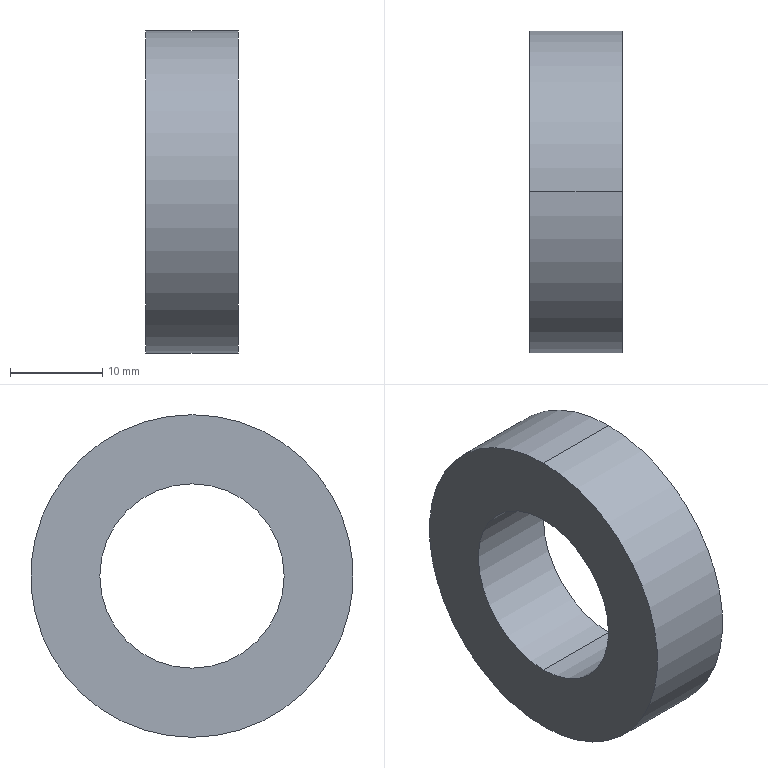Part | STEP file | urws35_20_10_2_03 | 1 solid | 6 faces | box 10 x 35 x 35 mm | volume 6480 mm3 | cylinder 4 | plane 2 | commonest cylinder face diameters 20 x2 35 x2
STEP:
#1=CARTESIAN_POINT('',(0.,0.,0.));
#2=DIRECTION('',(0.,0.,1.));
#3=DIRECTION('',(1.,0.,0.));
#4=AXIS2_PLACEMENT_3D('',#1,#2,#3);
#5=CARTESIAN_POINT('',(0.,0.,-17.5));
#6=VERTEX_POINT('',#5);
#7=CARTESIAN_POINT('',(0.,0.,17.5));
#8=VERTEX_POINT('',#7);
#9=CARTESIAN_POINT('',(0.,0.,0.));
#10=DIRECTION('',(1.,0.,0.));
#11=DIRECTION('',(0.,0.,-1.));
#12=AXIS2_PLACEMENT_3D('',#9,#10,#11);
#13=CIRCLE('',#12,17.5);
#14=CARTESIAN_POINT('',(5.,0.,0.));
#15=DIRECTION('',(1.,0.,0.));
#16=DIRECTION('',(0.,0.,-1.));
#17=AXIS2_PLACEMENT_3D('',#14,#15,#16);
#18=CYLINDRICAL_SURFACE('',#17,17.5);
#19=CARTESIAN_POINT('',(0.,-5.));
#20=DIRECTION('',(1.,0.));
#21=VECTOR('',#20,1.);
#22=LINE('',#19,#21);
#23=(GEOMETRIC_REPRESENTATION_CONTEXT(2)PARAMETRIC_REPRESENTATION_CONTEXT()REPRESENTATION_CONTEXT('',''));
#24=DEFINITIONAL_REPRESENTATION('',(#22),#23);
#25=PCURVE('',#18,#24);
#26=CARTESIAN_POINT('',(0.,8.75,0.));
#27=DIRECTION('',(-1.,0.,0.));
#28=DIRECTION('',(0.,0.,1.));
#29=AXIS2_PLACEMENT_3D('',#26,#27,#28);
#30=PLANE('',#29);
#31=CARTESIAN_POINT('',(-17.5,-8.75));
#32=CARTESIAN_POINT('',(-17.5,21.561));
#33=CARTESIAN_POINT('',(8.75,6.405));
#34=CARTESIAN_POINT('',(35.,-8.75));
#35=CARTESIAN_POINT('',(8.75,-23.905));
#36=CARTESIAN_POINT('',(-17.5,-39.061));
#37=CARTESIAN_POINT('',(-17.5,-8.75));
#38=(BOUNDED_CURVE()B_SPLINE_CURVE(2,(#31,#32,#33,#34,#35,#36,#37),.UNSPECIFIED.,.T.,.F.)B_SPLINE_CURVE_WITH_KNOTS((1,2,2,2,2,1),(-2.094,0.,2.094,4.189,6.283,8.378),.UNSPECIFIED.)CURVE()GEOMETRIC_REPRESENTATION_ITEM()RATIONAL_B_SPLINE_CURVE((1.,0.5,1.,0.5,1.,0.5,1.))REPRESENTATION_ITEM(''));
#39=(GEOMETRIC_REPRESENTATION_CONTEXT(2)PARAMETRIC_REPRESENTATION_CONTEXT()REPRESENTATION_CONTEXT('',''));
#40=DEFINITIONAL_REPRESENTATION('',(#38),#39);
#41=PCURVE('',#30,#40);
#42=SURFACE_CURVE('',#13,(#25,#41),.PCURVE_S1.);
#43=EDGE_CURVE('',#6,#8,#42,.T.);
#44=ORIENTED_EDGE('',*,*,#43,.T.);
#45=CARTESIAN_POINT('',(10.,0.,17.5));
#46=VERTEX_POINT('',#45);
#47=CARTESIAN_POINT('',(5.,0.,17.5));
#48=DIRECTION('',(1.,0.,0.));
#49=VECTOR('',#48,1.);
#50=LINE('',#47,#49);
#51=CARTESIAN_POINT('',(3.142,0.));
#52=DIRECTION('',(0.,1.));
#53=VECTOR('',#52,1.);
#54=LINE('',#51,#53);
#55=(GEOMETRIC_REPRESENTATION_CONTEXT(2)PARAMETRIC_REPRESENTATION_CONTEXT()REPRESENTATION_CONTEXT('',''));
#56=DEFINITIONAL_REPRESENTATION('',(#54),#55);
#57=PCURVE('',#18,#56);
#58=CARTESIAN_POINT('',(5.,0.,0.));
#59=DIRECTION('',(1.,0.,0.));
#60=DIRECTION('',(0.,0.,-1.));
#61=AXIS2_PLACEMENT_3D('',#58,#59,#60);
#62=CYLINDRICAL_SURFACE('',#61,17.5);
#63=CARTESIAN_POINT('',(3.142,0.));
#64=DIRECTION('',(0.,1.));
#65=VECTOR('',#64,1.);
#66=LINE('',#63,#65);
#67=(GEOMETRIC_REPRESENTATION_CONTEXT(2)PARAMETRIC_REPRESENTATION_CONTEXT()REPRESENTATION_CONTEXT('',''));
#68=DEFINITIONAL_REPRESENTATION('',(#66),#67);
#69=PCURVE('',#62,#68);
#70=SURFACE_CURVE('',#50,(#57,#69),.PCURVE_S1.);
#71=EDGE_CURVE('',#8,#46,#70,.T.);
#72=ORIENTED_EDGE('',*,*,#71,.T.);
#73=CARTESIAN_POINT('',(10.,0.,-17.5));
#74=VERTEX_POINT('',#73);
#75=CARTESIAN_POINT('',(10.,0.,0.));
#76=DIRECTION('',(1.,0.,0.));
#77=DIRECTION('',(0.,0.,-1.));
#78=AXIS2_PLACEMENT_3D('',#75,#76,#77);
#79=CIRCLE('',#78,17.5);
#80=CARTESIAN_POINT('',(0.,5.));
#81=DIRECTION('',(1.,0.));
#82=VECTOR('',#81,1.);
#83=LINE('',#80,#82);
#84=(GEOMETRIC_REPRESENTATION_CONTEXT(2)PARAMETRIC_REPRESENTATION_CONTEXT()REPRESENTATION_CONTEXT('',''));
#85=DEFINITIONAL_REPRESENTATION('',(#83),#84);
#86=PCURVE('',#18,#85);
#87=CARTESIAN_POINT('',(10.,8.75,0.));
#88=DIRECTION('',(1.,0.,0.));
#89=DIRECTION('',(0.,0.,-1.));
#90=AXIS2_PLACEMENT_3D('',#87,#88,#89);
#91=PLANE('',#90);
#92=CARTESIAN_POINT('',(0.,-8.75));
#93=DIRECTION('',(1.,0.));
#94=AXIS2_PLACEMENT_2D('',#92,#93);
#95=CIRCLE('',#94,17.5);
#96=(GEOMETRIC_REPRESENTATION_CONTEXT(2)PARAMETRIC_REPRESENTATION_CONTEXT()REPRESENTATION_CONTEXT('',''));
#97=DEFINITIONAL_REPRESENTATION('',(#95),#96);
#98=PCURVE('',#91,#97);
#99=SURFACE_CURVE('',#79,(#86,#98),.PCURVE_S1.);
#100=EDGE_CURVE('',#74,#46,#99,.T.);
#101=ORIENTED_EDGE('',*,*,#100,.F.);
#102=CARTESIAN_POINT('',(5.,0.,-17.5));
#103=DIRECTION('',(1.,0.,0.));
#104=VECTOR('',#103,1.);
#105=LINE('',#102,#104);
#106=CARTESIAN_POINT('',(0.,0.));
#107=DIRECTION('',(0.,1.));
#108=VECTOR('',#107,1.);
#109=LINE('',#106,#108);
#110=(GEOMETRIC_REPRESENTATION_CONTEXT(2)PARAMETRIC_REPRESENTATION_CONTEXT()REPRESENTATION_CONTEXT('',''));
#111=DEFINITIONAL_REPRESENTATION('',(#109),#110);
#112=PCURVE('',#18,#111);
#113=CARTESIAN_POINT('',(6.283,0.));
#114=DIRECTION('',(0.,1.));
#115=VECTOR('',#114,1.);
#116=LINE('',#113,#115);
#117=(GEOMETRIC_REPRESENTATION_CONTEXT(2)PARAMETRIC_REPRESENTATION_CONTEXT()REPRESENTATION_CONTEXT('',''));
#118=DEFINITIONAL_REPRESENTATION('',(#116),#117);
#119=PCURVE('',#62,#118);
#120=SURFACE_CURVE('',#105,(#112,#119),.PCURVE_S1.);
#121=EDGE_CURVE('',#6,#74,#120,.T.);
#122=ORIENTED_EDGE('',*,*,#121,.F.);
#123=EDGE_LOOP('',(#44,#72,#101,#122));
#124=FACE_BOUND('',#123,.T.);
#125=ADVANCED_FACE('',(#124),#18,.T.);
#126=CARTESIAN_POINT('',(10.,0.,10.));
#127=VERTEX_POINT('',#126);
#128=CARTESIAN_POINT('',(0.,0.,10.));
#129=VERTEX_POINT('',#128);
#130=CARTESIAN_POINT('',(0.,0.,10.));
#131=DIRECTION('',(-1.,0.,0.));
#132=VECTOR('',#131,1.);
#133=LINE('',#130,#132);
#134=CARTESIAN_POINT('',(0.,0.,0.));
#135=DIRECTION('',(-1.,0.,0.));
#136=DIRECTION('',(0.,0.,1.));
#137=AXIS2_PLACEMENT_3D('',#134,#135,#136);
#138=CYLINDRICAL_SURFACE('',#137,10.);
#139=CARTESIAN_POINT('',(6.283,0.));
#140=DIRECTION('',(0.,1.));
#141=VECTOR('',#140,1.);
#142=LINE('',#139,#141);
#143=(GEOMETRIC_REPRESENTATION_CONTEXT(2)PARAMETRIC_REPRESENTATION_CONTEXT()REPRESENTATION_CONTEXT('',''));
#144=DEFINITIONAL_REPRESENTATION('',(#142),#143);
#145=PCURVE('',#138,#144);
#146=CARTESIAN_POINT('',(0.,0.,0.));
#147=DIRECTION('',(-1.,0.,0.));
#148=DIRECTION('',(0.,0.,1.));
#149=AXIS2_PLACEMENT_3D('',#146,#147,#148);
#150=CYLINDRICAL_SURFACE('',#149,10.);
#151=CARTESIAN_POINT('',(0.,0.));
#152=DIRECTION('',(0.,1.));
#153=VECTOR('',#152,1.);
#154=LINE('',#151,#153);
#155=(GEOMETRIC_REPRESENTATION_CONTEXT(2)PARAMETRIC_REPRESENTATION_CONTEXT()REPRESENTATION_CONTEXT('',''));
#156=DEFINITIONAL_REPRESENTATION('',(#154),#155);
#157=PCURVE('',#150,#156);
#158=SURFACE_CURVE('',#133,(#145,#157),.PCURVE_S1.);
#159=EDGE_CURVE('',#127,#129,#158,.T.);
#160=ORIENTED_EDGE('',*,*,#159,.T.);
#161=CARTESIAN_POINT('',(0.,0.,-10.));
#162=VERTEX_POINT('',#161);
#163=CARTESIAN_POINT('',(0.,0.,0.));
#164=DIRECTION('',(1.,0.,0.));
#165=DIRECTION('',(0.,0.,1.));
#166=AXIS2_PLACEMENT_3D('',#163,#164,#165);
#167=CIRCLE('',#166,10.);
#168=CARTESIAN_POINT('',(6.283,0.));
#169=DIRECTION('',(-1.,0.));
#170=VECTOR('',#169,1.);
#171=LINE('',#168,#170);
#172=(GEOMETRIC_REPRESENTATION_CONTEXT(2)PARAMETRIC_REPRESENTATION_CONTEXT()REPRESENTATION_CONTEXT('',''));
#173=DEFINITIONAL_REPRESENTATION('',(#171),#172);
#174=PCURVE('',#138,#173);
#175=CARTESIAN_POINT('',(10.,-8.75));
#176=CARTESIAN_POINT('',(10.,-26.071));
#177=CARTESIAN_POINT('',(-5.,-17.41));
#178=CARTESIAN_POINT('',(-20.,-8.75));
#179=CARTESIAN_POINT('',(-5.,-0.08975));
#180=CARTESIAN_POINT('',(10.,8.571));
#181=CARTESIAN_POINT('',(10.,-8.75));
#182=(BOUNDED_CURVE()B_SPLINE_CURVE(2,(#175,#176,#177,#178,#179,#180,#181),.UNSPECIFIED.,.T.,.F.)B_SPLINE_CURVE_WITH_KNOTS((1,2,2,2,2,1),(-2.094,0.,2.094,4.189,6.283,8.378),.UNSPECIFIED.)CURVE()GEOMETRIC_REPRESENTATION_ITEM()RATIONAL_B_SPLINE_CURVE((1.,0.5,1.,0.5,1.,0.5,1.))REPRESENTATION_ITEM(''));
#183=(GEOMETRIC_REPRESENTATION_CONTEXT(2)PARAMETRIC_REPRESENTATION_CONTEXT()REPRESENTATION_CONTEXT('',''));
#184=DEFINITIONAL_REPRESENTATION('',(#182),#183);
#185=PCURVE('',#30,#184);
#186=SURFACE_CURVE('',#167,(#174,#185),.PCURVE_S1.);
#187=EDGE_CURVE('',#129,#162,#186,.T.);
#188=ORIENTED_EDGE('',*,*,#187,.T.);
#189=CARTESIAN_POINT('',(10.,0.,-10.));
#190=VERTEX_POINT('',#189);
#191=CARTESIAN_POINT('',(0.,0.,-10.));
#192=DIRECTION('',(-1.,0.,0.));
#193=VECTOR('',#192,1.);
#194=LINE('',#191,#193);
#195=CARTESIAN_POINT('',(3.142,0.));
#196=DIRECTION('',(0.,1.));
#197=VECTOR('',#196,1.);
#198=LINE('',#195,#197);
#199=(GEOMETRIC_REPRESENTATION_CONTEXT(2)PARAMETRIC_REPRESENTATION_CONTEXT()REPRESENTATION_CONTEXT('',''));
#200=DEFINITIONAL_REPRESENTATION('',(#198),#199);
#201=PCURVE('',#138,#200);
#202=CARTESIAN_POINT('',(3.142,0.));
#203=DIRECTION('',(0.,1.));
#204=VECTOR('',#203,1.);
#205=LINE('',#202,#204);
#206=(GEOMETRIC_REPRESENTATION_CONTEXT(2)PARAMETRIC_REPRESENTATION_CONTEXT()REPRESENTATION_CONTEXT('',''));
#207=DEFINITIONAL_REPRESENTATION('',(#205),#206);
#208=PCURVE('',#150,#207);
#209=SURFACE_CURVE('',#194,(#201,#208),.PCURVE_S1.);
#210=EDGE_CURVE('',#190,#162,#209,.T.);
#211=ORIENTED_EDGE('',*,*,#210,.F.);
#212=CARTESIAN_POINT('',(10.,0.,0.));
#213=DIRECTION('',(-1.,0.,0.));
#214=DIRECTION('',(0.,0.,1.));
#215=AXIS2_PLACEMENT_3D('',#212,#213,#214);
#216=CIRCLE('',#215,10.);
#217=CARTESIAN_POINT('',(0.,-10.));
#218=DIRECTION('',(1.,0.));
#219=VECTOR('',#218,1.);
#220=LINE('',#217,#219);
#221=(GEOMETRIC_REPRESENTATION_CONTEXT(2)PARAMETRIC_REPRESENTATION_CONTEXT()REPRESENTATION_CONTEXT('',''));
#222=DEFINITIONAL_REPRESENTATION('',(#220),#221);
#223=PCURVE('',#138,#222);
#224=CARTESIAN_POINT('',(-10.,-8.75));
#225=CARTESIAN_POINT('',(-10.,8.571));
#226=CARTESIAN_POINT('',(5.,-0.08975));
#227=CARTESIAN_POINT('',(20.,-8.75));
#228=CARTESIAN_POINT('',(5.,-17.41));
#229=CARTESIAN_POINT('',(-10.,-26.071));
#230=CARTESIAN_POINT('',(-10.,-8.75));
#231=(BOUNDED_CURVE()B_SPLINE_CURVE(2,(#224,#225,#226,#227,#228,#229,#230),.UNSPECIFIED.,.T.,.F.)B_SPLINE_CURVE_WITH_KNOTS((1,2,2,2,2,1),(-2.094,0.,2.094,4.189,6.283,8.378),.UNSPECIFIED.)CURVE()GEOMETRIC_REPRESENTATION_ITEM()RATIONAL_B_SPLINE_CURVE((1.,0.5,1.,0.5,1.,0.5,1.))REPRESENTATION_ITEM(''));
#232=(GEOMETRIC_REPRESENTATION_CONTEXT(2)PARAMETRIC_REPRESENTATION_CONTEXT()REPRESENTATION_CONTEXT('',''));
#233=DEFINITIONAL_REPRESENTATION('',(#231),#232);
#234=PCURVE('',#91,#233);
#235=SURFACE_CURVE('',#216,(#223,#234),.PCURVE_S1.);
#236=EDGE_CURVE('',#190,#127,#235,.T.);
#237=ORIENTED_EDGE('',*,*,#236,.T.);
#238=EDGE_LOOP('',(#160,#188,#211,#237));
#239=FACE_BOUND('',#238,.F.);
#240=ADVANCED_FACE('',(#239),#138,.F.);
#241=ORIENTED_EDGE('',*,*,#100,.T.);
#242=CARTESIAN_POINT('',(10.,0.,0.));
#243=DIRECTION('',(1.,0.,0.));
#244=DIRECTION('',(0.,0.,-1.));
#245=AXIS2_PLACEMENT_3D('',#242,#243,#244);
#246=CIRCLE('',#245,17.5);
#247=CARTESIAN_POINT('',(0.,-8.75));
#248=DIRECTION('',(1.,0.));
#249=AXIS2_PLACEMENT_2D('',#247,#248);
#250=CIRCLE('',#249,17.5);
#251=(GEOMETRIC_REPRESENTATION_CONTEXT(2)PARAMETRIC_REPRESENTATION_CONTEXT()REPRESENTATION_CONTEXT('',''));
#252=DEFINITIONAL_REPRESENTATION('',(#250),#251);
#253=PCURVE('',#91,#252);
#254=CARTESIAN_POINT('',(0.,5.));
#255=DIRECTION('',(1.,0.));
#256=VECTOR('',#255,1.);
#257=LINE('',#254,#256);
#258=(GEOMETRIC_REPRESENTATION_CONTEXT(2)PARAMETRIC_REPRESENTATION_CONTEXT()REPRESENTATION_CONTEXT('',''));
#259=DEFINITIONAL_REPRESENTATION('',(#257),#258);
#260=PCURVE('',#62,#259);
#261=SURFACE_CURVE('',#246,(#253,#260),.PCURVE_S1.);
#262=EDGE_CURVE('',#46,#74,#261,.T.);
#263=ORIENTED_EDGE('',*,*,#262,.T.);
#264=EDGE_LOOP('',(#241,#263));
#265=FACE_BOUND('',#264,.T.);
#266=CARTESIAN_POINT('',(10.,0.,0.));
#267=DIRECTION('',(-1.,0.,0.));
#268=DIRECTION('',(0.,0.,1.));
#269=AXIS2_PLACEMENT_3D('',#266,#267,#268);
#270=CIRCLE('',#269,10.);
#271=CARTESIAN_POINT('',(-10.,-8.75));
#272=CARTESIAN_POINT('',(-10.,8.571));
#273=CARTESIAN_POINT('',(5.,-0.08975));
#274=CARTESIAN_POINT('',(20.,-8.75));
#275=CARTESIAN_POINT('',(5.,-17.41));
#276=CARTESIAN_POINT('',(-10.,-26.071));
#277=CARTESIAN_POINT('',(-10.,-8.75));
#278=(BOUNDED_CURVE()B_SPLINE_CURVE(2,(#271,#272,#273,#274,#275,#276,#277),.UNSPECIFIED.,.T.,.F.)B_SPLINE_CURVE_WITH_KNOTS((1,2,2,2,2,1),(-2.094,0.,2.094,4.189,6.283,8.378),.UNSPECIFIED.)CURVE()GEOMETRIC_REPRESENTATION_ITEM()RATIONAL_B_SPLINE_CURVE((1.,0.5,1.,0.5,1.,0.5,1.))REPRESENTATION_ITEM(''));
#279=(GEOMETRIC_REPRESENTATION_CONTEXT(2)PARAMETRIC_REPRESENTATION_CONTEXT()REPRESENTATION_CONTEXT('',''));
#280=DEFINITIONAL_REPRESENTATION('',(#278),#279);
#281=PCURVE('',#91,#280);
#282=CARTESIAN_POINT('',(0.,-10.));
#283=DIRECTION('',(1.,0.));
#284=VECTOR('',#283,1.);
#285=LINE('',#282,#284);
#286=(GEOMETRIC_REPRESENTATION_CONTEXT(2)PARAMETRIC_REPRESENTATION_CONTEXT()REPRESENTATION_CONTEXT('',''));
#287=DEFINITIONAL_REPRESENTATION('',(#285),#286);
#288=PCURVE('',#150,#287);
#289=SURFACE_CURVE('',#270,(#281,#288),.PCURVE_S1.);
#290=EDGE_CURVE('',#127,#190,#289,.T.);
#291=ORIENTED_EDGE('',*,*,#290,.T.);
#292=ORIENTED_EDGE('',*,*,#236,.T.);
#293=EDGE_LOOP('',(#291,#292));
#294=FACE_BOUND('',#293,.T.);
#295=ADVANCED_FACE('',(#265,#294),#91,.T.);
#296=ORIENTED_EDGE('',*,*,#71,.F.);
#297=CARTESIAN_POINT('',(0.,0.,0.));
#298=DIRECTION('',(1.,0.,0.));
#299=DIRECTION('',(0.,0.,-1.));
#300=AXIS2_PLACEMENT_3D('',#297,#298,#299);
#301=CIRCLE('',#300,17.5);
#302=CARTESIAN_POINT('',(0.,-5.));
#303=DIRECTION('',(1.,0.));
#304=VECTOR('',#303,1.);
#305=LINE('',#302,#304);
#306=(GEOMETRIC_REPRESENTATION_CONTEXT(2)PARAMETRIC_REPRESENTATION_CONTEXT()REPRESENTATION_CONTEXT('',''));
#307=DEFINITIONAL_REPRESENTATION('',(#305),#306);
#308=PCURVE('',#62,#307);
#309=CARTESIAN_POINT('',(-17.5,-8.75));
#310=CARTESIAN_POINT('',(-17.5,21.561));
#311=CARTESIAN_POINT('',(8.75,6.405));
#312=CARTESIAN_POINT('',(35.,-8.75));
#313=CARTESIAN_POINT('',(8.75,-23.905));
#314=CARTESIAN_POINT('',(-17.5,-39.061));
#315=CARTESIAN_POINT('',(-17.5,-8.75));
#316=(BOUNDED_CURVE()B_SPLINE_CURVE(2,(#309,#310,#311,#312,#313,#314,#315),.UNSPECIFIED.,.T.,.F.)B_SPLINE_CURVE_WITH_KNOTS((1,2,2,2,2,1),(-2.094,0.,2.094,4.189,6.283,8.378),.UNSPECIFIED.)CURVE()GEOMETRIC_REPRESENTATION_ITEM()RATIONAL_B_SPLINE_CURVE((1.,0.5,1.,0.5,1.,0.5,1.))REPRESENTATION_ITEM(''));
#317=(GEOMETRIC_REPRESENTATION_CONTEXT(2)PARAMETRIC_REPRESENTATION_CONTEXT()REPRESENTATION_CONTEXT('',''));
#318=DEFINITIONAL_REPRESENTATION('',(#316),#317);
#319=PCURVE('',#30,#318);
#320=SURFACE_CURVE('',#301,(#308,#319),.PCURVE_S1.);
#321=EDGE_CURVE('',#8,#6,#320,.T.);
#322=ORIENTED_EDGE('',*,*,#321,.T.);
#323=ORIENTED_EDGE('',*,*,#121,.T.);
#324=ORIENTED_EDGE('',*,*,#262,.F.);
#325=EDGE_LOOP('',(#296,#322,#323,#324));
#326=FACE_BOUND('',#325,.T.);
#327=ADVANCED_FACE('',(#326),#62,.T.);
#328=CARTESIAN_POINT('',(0.,0.,0.));
#329=DIRECTION('',(1.,0.,0.));
#330=DIRECTION('',(0.,0.,1.));
#331=AXIS2_PLACEMENT_3D('',#328,#329,#330);
#332=CIRCLE('',#331,10.);
#333=CARTESIAN_POINT('',(6.283,0.));
#334=DIRECTION('',(-1.,0.));
#335=VECTOR('',#334,1.);
#336=LINE('',#333,#335);
#337=(GEOMETRIC_REPRESENTATION_CONTEXT(2)PARAMETRIC_REPRESENTATION_CONTEXT()REPRESENTATION_CONTEXT('',''));
#338=DEFINITIONAL_REPRESENTATION('',(#336),#337);
#339=PCURVE('',#150,#338);
#340=CARTESIAN_POINT('',(10.,-8.75));
#341=CARTESIAN_POINT('',(10.,-26.071));
#342=CARTESIAN_POINT('',(-5.,-17.41));
#343=CARTESIAN_POINT('',(-20.,-8.75));
#344=CARTESIAN_POINT('',(-5.,-0.08975));
#345=CARTESIAN_POINT('',(10.,8.571));
#346=CARTESIAN_POINT('',(10.,-8.75));
#347=(BOUNDED_CURVE()B_SPLINE_CURVE(2,(#340,#341,#342,#343,#344,#345,#346),.UNSPECIFIED.,.T.,.F.)B_SPLINE_CURVE_WITH_KNOTS((1,2,2,2,2,1),(-2.094,0.,2.094,4.189,6.283,8.378),.UNSPECIFIED.)CURVE()GEOMETRIC_REPRESENTATION_ITEM()RATIONAL_B_SPLINE_CURVE((1.,0.5,1.,0.5,1.,0.5,1.))REPRESENTATION_ITEM(''));
#348=(GEOMETRIC_REPRESENTATION_CONTEXT(2)PARAMETRIC_REPRESENTATION_CONTEXT()REPRESENTATION_CONTEXT('',''));
#349=DEFINITIONAL_REPRESENTATION('',(#347),#348);
#350=PCURVE('',#30,#349);
#351=SURFACE_CURVE('',#332,(#339,#350),.PCURVE_S1.);
#352=EDGE_CURVE('',#162,#129,#351,.T.);
#353=ORIENTED_EDGE('',*,*,#352,.T.);
#354=ORIENTED_EDGE('',*,*,#159,.F.);
#355=ORIENTED_EDGE('',*,*,#290,.T.);
#356=ORIENTED_EDGE('',*,*,#210,.T.);
#357=EDGE_LOOP('',(#353,#354,#355,#356));
#358=FACE_BOUND('',#357,.F.);
#359=ADVANCED_FACE('',(#358),#150,.F.);
#360=ORIENTED_EDGE('',*,*,#43,.F.);
#361=ORIENTED_EDGE('',*,*,#321,.F.);
#362=EDGE_LOOP('',(#360,#361));
#363=FACE_BOUND('',#362,.T.);
#364=ORIENTED_EDGE('',*,*,#187,.T.);
#365=ORIENTED_EDGE('',*,*,#352,.T.);
#366=EDGE_LOOP('',(#364,#365));
#367=FACE_BOUND('',#366,.T.);
#368=ADVANCED_FACE('',(#363,#367),#30,.T.);
#369=CLOSED_SHELL('',(#125,#240,#295,#327,#359,#368));
#370=MANIFOLD_SOLID_BREP('',#369);
#371=(LENGTH_UNIT()NAMED_UNIT(*)SI_UNIT(.MILLI.,.METRE.));
#372=UNCERTAINTY_MEASURE_WITH_UNIT(LENGTH_MEASURE(0.0000001),#371,'','');
#373=(NAMED_UNIT(*)PLANE_ANGLE_UNIT()SI_UNIT($,.RADIAN.));
#374=(NAMED_UNIT(*)SI_UNIT($,.STERADIAN.)SOLID_ANGLE_UNIT());
#375=(GEOMETRIC_REPRESENTATION_CONTEXT(3)GLOBAL_UNCERTAINTY_ASSIGNED_CONTEXT((#372))GLOBAL_UNIT_ASSIGNED_CONTEXT((#371,#373,#374))REPRESENTATION_CONTEXT('',''));
#376=ADVANCED_BREP_SHAPE_REPRESENTATION('',(#4,#370),#375);